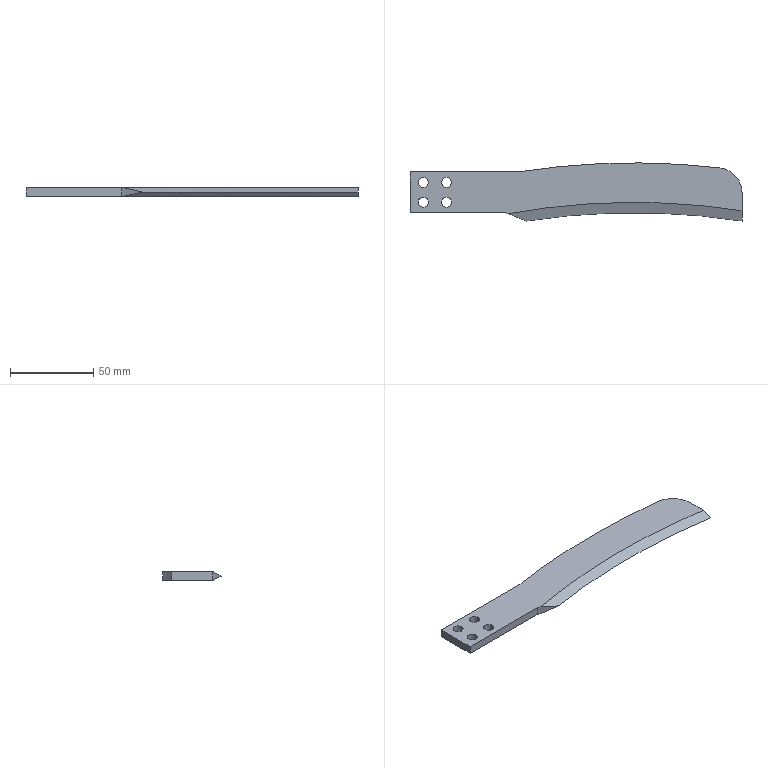Part | STEP file | Cut-off blade | 1 solid | 19 faces | box 200 x 35.06 x 5 mm | volume 25538 mm3 | cylinder 10 | plane 7 | cone 2 | commonest cylinder face diameters 6 x8 30 x1 900 x1
STEP:
#1=CARTESIAN_POINT('',(-51.,23.319,0.));
#2=VERTEX_POINT('',#1);
#3=CARTESIAN_POINT('',(-45.,23.319,0.));
#4=VERTEX_POINT('',#3);
#5=CARTESIAN_POINT('',(-48.,23.319,0.));
#6=DIRECTION('',(0.,0.,1.));
#7=DIRECTION('',(1.,0.,0.));
#8=AXIS2_PLACEMENT_3D('',#5,#6,#7);
#9=CIRCLE('',#8,3.);
#10=EDGE_CURVE('',#2,#4,#9,.T.);
#11=ORIENTED_EDGE('',*,*,#10,.F.);
#12=CARTESIAN_POINT('',(-51.,23.319,5.));
#13=VERTEX_POINT('',#12);
#14=CARTESIAN_POINT('',(-51.,23.319,0.));
#15=DIRECTION('',(0.,0.,1.));
#16=VECTOR('',#15,1000.);
#17=LINE('',#14,#16);
#18=EDGE_CURVE('',#2,#13,#17,.T.);
#19=ORIENTED_EDGE('',*,*,#18,.T.);
#20=CARTESIAN_POINT('',(-45.,23.319,5.));
#21=VERTEX_POINT('',#20);
#22=CARTESIAN_POINT('',(-48.,23.319,5.));
#23=DIRECTION('',(0.,0.,1.));
#24=DIRECTION('',(1.,0.,0.));
#25=AXIS2_PLACEMENT_3D('',#22,#23,#24);
#26=CIRCLE('',#25,3.);
#27=EDGE_CURVE('',#13,#21,#26,.T.);
#28=ORIENTED_EDGE('',*,*,#27,.T.);
#29=CARTESIAN_POINT('',(-45.,23.319,0.));
#30=DIRECTION('',(0.,0.,1.));
#31=VECTOR('',#30,1000.);
#32=LINE('',#29,#31);
#33=EDGE_CURVE('',#4,#21,#32,.T.);
#34=ORIENTED_EDGE('',*,*,#33,.F.);
#35=EDGE_LOOP('',(#11,#19,#28,#34));
#36=FACE_OUTER_BOUND('',#35,.T.);
#37=CARTESIAN_POINT('',(-48.,23.319,0.));
#38=DIRECTION('',(0.,0.,1.));
#39=DIRECTION('',(1.,0.,0.));
#40=AXIS2_PLACEMENT_3D('',#37,#38,#39);
#41=CYLINDRICAL_SURFACE('',#40,3.);
#42=ADVANCED_FACE('',(#36),#41,.F.);
#43=CARTESIAN_POINT('',(-51.,11.319,0.));
#44=VERTEX_POINT('',#43);
#45=CARTESIAN_POINT('',(-45.,11.319,0.));
#46=VERTEX_POINT('',#45);
#47=CARTESIAN_POINT('',(-48.,11.319,0.));
#48=DIRECTION('',(0.,0.,1.));
#49=DIRECTION('',(-1.,0.,0.));
#50=AXIS2_PLACEMENT_3D('',#47,#48,#49);
#51=CIRCLE('',#50,3.);
#52=EDGE_CURVE('',#44,#46,#51,.T.);
#53=ORIENTED_EDGE('',*,*,#52,.F.);
#54=CARTESIAN_POINT('',(-51.,11.319,5.));
#55=VERTEX_POINT('',#54);
#56=CARTESIAN_POINT('',(-51.,11.319,0.));
#57=DIRECTION('',(0.,0.,1.));
#58=VECTOR('',#57,1000.);
#59=LINE('',#56,#58);
#60=EDGE_CURVE('',#44,#55,#59,.T.);
#61=ORIENTED_EDGE('',*,*,#60,.T.);
#62=CARTESIAN_POINT('',(-45.,11.319,5.));
#63=VERTEX_POINT('',#62);
#64=CARTESIAN_POINT('',(-48.,11.319,5.));
#65=DIRECTION('',(0.,0.,1.));
#66=DIRECTION('',(-1.,0.,0.));
#67=AXIS2_PLACEMENT_3D('',#64,#65,#66);
#68=CIRCLE('',#67,3.);
#69=EDGE_CURVE('',#55,#63,#68,.T.);
#70=ORIENTED_EDGE('',*,*,#69,.T.);
#71=CARTESIAN_POINT('',(-45.,11.319,0.));
#72=DIRECTION('',(0.,0.,1.));
#73=VECTOR('',#72,1000.);
#74=LINE('',#71,#73);
#75=EDGE_CURVE('',#46,#63,#74,.T.);
#76=ORIENTED_EDGE('',*,*,#75,.F.);
#77=EDGE_LOOP('',(#53,#61,#70,#76));
#78=FACE_OUTER_BOUND('',#77,.T.);
#79=CARTESIAN_POINT('',(-48.,11.319,0.));
#80=DIRECTION('',(0.,0.,1.));
#81=DIRECTION('',(1.,0.,0.));
#82=AXIS2_PLACEMENT_3D('',#79,#80,#81);
#83=CYLINDRICAL_SURFACE('',#82,3.);
#84=ADVANCED_FACE('',(#78),#83,.F.);
#85=CARTESIAN_POINT('',(-65.,11.319,0.));
#86=VERTEX_POINT('',#85);
#87=CARTESIAN_POINT('',(-59.,11.319,0.));
#88=VERTEX_POINT('',#87);
#89=CARTESIAN_POINT('',(-62.,11.319,0.));
#90=DIRECTION('',(0.,0.,1.));
#91=DIRECTION('',(-1.,0.,0.));
#92=AXIS2_PLACEMENT_3D('',#89,#90,#91);
#93=CIRCLE('',#92,3.);
#94=EDGE_CURVE('',#86,#88,#93,.T.);
#95=ORIENTED_EDGE('',*,*,#94,.F.);
#96=CARTESIAN_POINT('',(-65.,11.319,5.));
#97=VERTEX_POINT('',#96);
#98=CARTESIAN_POINT('',(-65.,11.319,0.));
#99=DIRECTION('',(0.,0.,1.));
#100=VECTOR('',#99,1000.);
#101=LINE('',#98,#100);
#102=EDGE_CURVE('',#86,#97,#101,.T.);
#103=ORIENTED_EDGE('',*,*,#102,.T.);
#104=CARTESIAN_POINT('',(-59.,11.319,5.));
#105=VERTEX_POINT('',#104);
#106=CARTESIAN_POINT('',(-62.,11.319,5.));
#107=DIRECTION('',(0.,0.,1.));
#108=DIRECTION('',(-1.,0.,0.));
#109=AXIS2_PLACEMENT_3D('',#106,#107,#108);
#110=CIRCLE('',#109,3.);
#111=EDGE_CURVE('',#97,#105,#110,.T.);
#112=ORIENTED_EDGE('',*,*,#111,.T.);
#113=CARTESIAN_POINT('',(-59.,11.319,0.));
#114=DIRECTION('',(0.,0.,1.));
#115=VECTOR('',#114,1000.);
#116=LINE('',#113,#115);
#117=EDGE_CURVE('',#88,#105,#116,.T.);
#118=ORIENTED_EDGE('',*,*,#117,.F.);
#119=EDGE_LOOP('',(#95,#103,#112,#118));
#120=FACE_OUTER_BOUND('',#119,.T.);
#121=CARTESIAN_POINT('',(-62.,11.319,0.));
#122=DIRECTION('',(0.,0.,1.));
#123=DIRECTION('',(1.,0.,0.));
#124=AXIS2_PLACEMENT_3D('',#121,#122,#123);
#125=CYLINDRICAL_SURFACE('',#124,3.);
#126=ADVANCED_FACE('',(#120),#125,.F.);
#127=CARTESIAN_POINT('',(-65.,23.319,0.));
#128=VERTEX_POINT('',#127);
#129=CARTESIAN_POINT('',(-59.,23.319,0.));
#130=VERTEX_POINT('',#129);
#131=CARTESIAN_POINT('',(-62.,23.319,0.));
#132=DIRECTION('',(0.,0.,1.));
#133=DIRECTION('',(1.,0.,0.));
#134=AXIS2_PLACEMENT_3D('',#131,#132,#133);
#135=CIRCLE('',#134,3.);
#136=EDGE_CURVE('',#128,#130,#135,.T.);
#137=ORIENTED_EDGE('',*,*,#136,.F.);
#138=CARTESIAN_POINT('',(-65.,23.319,5.));
#139=VERTEX_POINT('',#138);
#140=CARTESIAN_POINT('',(-65.,23.319,0.));
#141=DIRECTION('',(0.,0.,1.));
#142=VECTOR('',#141,1000.);
#143=LINE('',#140,#142);
#144=EDGE_CURVE('',#128,#139,#143,.T.);
#145=ORIENTED_EDGE('',*,*,#144,.T.);
#146=CARTESIAN_POINT('',(-59.,23.319,5.));
#147=VERTEX_POINT('',#146);
#148=CARTESIAN_POINT('',(-62.,23.319,5.));
#149=DIRECTION('',(0.,0.,1.));
#150=DIRECTION('',(1.,0.,0.));
#151=AXIS2_PLACEMENT_3D('',#148,#149,#150);
#152=CIRCLE('',#151,3.);
#153=EDGE_CURVE('',#139,#147,#152,.T.);
#154=ORIENTED_EDGE('',*,*,#153,.T.);
#155=CARTESIAN_POINT('',(-59.,23.319,0.));
#156=DIRECTION('',(0.,0.,1.));
#157=VECTOR('',#156,1000.);
#158=LINE('',#155,#157);
#159=EDGE_CURVE('',#130,#147,#158,.T.);
#160=ORIENTED_EDGE('',*,*,#159,.F.);
#161=EDGE_LOOP('',(#137,#145,#154,#160));
#162=FACE_OUTER_BOUND('',#161,.T.);
#163=CARTESIAN_POINT('',(-62.,23.319,0.));
#164=DIRECTION('',(0.,0.,1.));
#165=DIRECTION('',(1.,0.,0.));
#166=AXIS2_PLACEMENT_3D('',#163,#164,#165);
#167=CYLINDRICAL_SURFACE('',#166,3.);
#168=ADVANCED_FACE('',(#162),#167,.F.);
#169=CARTESIAN_POINT('',(130.,6.262,0.));
#170=VERTEX_POINT('',#169);
#171=CARTESIAN_POINT('',(130.,17.177,0.));
#172=VERTEX_POINT('',#171);
#173=CARTESIAN_POINT('',(130.,0.,0.));
#174=DIRECTION('',(0.,1.,0.));
#175=VECTOR('',#174,1000.);
#176=LINE('',#173,#175);
#177=EDGE_CURVE('',#170,#172,#176,.T.);
#178=ORIENTED_EDGE('',*,*,#177,.T.);
#179=CARTESIAN_POINT('',(130.,17.177,5.));
#180=VERTEX_POINT('',#179);
#181=CARTESIAN_POINT('',(130.,17.177,5.));
#182=DIRECTION('',(0.,0.,1.));
#183=VECTOR('',#182,1000.);
#184=LINE('',#181,#183);
#185=EDGE_CURVE('',#172,#180,#184,.T.);
#186=ORIENTED_EDGE('',*,*,#185,.T.);
#187=CARTESIAN_POINT('',(130.,6.262,5.));
#188=VERTEX_POINT('',#187);
#189=CARTESIAN_POINT('',(130.,0.,5.));
#190=DIRECTION('',(0.,1.,0.));
#191=VECTOR('',#190,1000.);
#192=LINE('',#189,#191);
#193=EDGE_CURVE('',#188,#180,#192,.T.);
#194=ORIENTED_EDGE('',*,*,#193,.F.);
#195=CARTESIAN_POINT('',(130.,0.,2.5));
#196=VERTEX_POINT('',#195);
#197=CARTESIAN_POINT('',(130.,6.262,5.));
#198=CARTESIAN_POINT('',(130.,4.175,4.167));
#199=CARTESIAN_POINT('',(130.,2.087,3.333));
#200=CARTESIAN_POINT('',(130.,0.,2.5));
#201=B_SPLINE_CURVE_WITH_KNOTS('',3,(#197,#198,#199,#200),.UNSPECIFIED.,.F.,.F.,(4,4),(0.,0.006743),.UNSPECIFIED.);
#202=EDGE_CURVE('',#188,#196,#201,.T.);
#203=ORIENTED_EDGE('',*,*,#202,.T.);
#204=CARTESIAN_POINT('',(130.,0.,2.5));
#205=CARTESIAN_POINT('',(130.,2.087,1.667));
#206=CARTESIAN_POINT('',(130.,4.175,0.8335));
#207=CARTESIAN_POINT('',(130.,6.262,0.));
#208=B_SPLINE_CURVE_WITH_KNOTS('',3,(#204,#205,#206,#207),.UNSPECIFIED.,.F.,.F.,(4,4),(0.,0.006743),.UNSPECIFIED.);
#209=EDGE_CURVE('',#196,#170,#208,.T.);
#210=ORIENTED_EDGE('',*,*,#209,.T.);
#211=EDGE_LOOP('',(#178,#186,#194,#203,#210));
#212=FACE_OUTER_BOUND('',#211,.T.);
#213=CARTESIAN_POINT('',(130.,0.,5.));
#214=DIRECTION('',(-1.,0.,0.));
#215=DIRECTION('',(0.,0.,1.));
#216=AXIS2_PLACEMENT_3D('',#213,#214,#215);
#217=PLANE('',#216);
#218=ADVANCED_FACE('',(#212),#217,.F.);
#219=CARTESIAN_POINT('',(116.724,32.078,5.));
#220=VERTEX_POINT('',#219);
#221=CARTESIAN_POINT('',(-4.643,29.639,5.));
#222=VERTEX_POINT('',#221);
#223=CARTESIAN_POINT('',(65.,-414.94,5.));
#224=DIRECTION('',(0.,0.,1.));
#225=DIRECTION('',(-1.,0.,0.));
#226=AXIS2_PLACEMENT_3D('',#223,#224,#225);
#227=CIRCLE('',#226,450.);
#228=EDGE_CURVE('',#220,#222,#227,.T.);
#229=ORIENTED_EDGE('',*,*,#228,.F.);
#230=CARTESIAN_POINT('',(116.724,32.078,0.));
#231=VERTEX_POINT('',#230);
#232=CARTESIAN_POINT('',(116.724,32.078,5.));
#233=DIRECTION('',(0.,0.,-1.));
#234=VECTOR('',#233,1000.);
#235=LINE('',#232,#234);
#236=EDGE_CURVE('',#220,#231,#235,.T.);
#237=ORIENTED_EDGE('',*,*,#236,.T.);
#238=CARTESIAN_POINT('',(-4.643,29.639,0.));
#239=VERTEX_POINT('',#238);
#240=CARTESIAN_POINT('',(65.,-414.94,0.));
#241=DIRECTION('',(0.,0.,1.));
#242=DIRECTION('',(-1.,0.,0.));
#243=AXIS2_PLACEMENT_3D('',#240,#241,#242);
#244=CIRCLE('',#243,450.);
#245=EDGE_CURVE('',#231,#239,#244,.T.);
#246=ORIENTED_EDGE('',*,*,#245,.T.);
#247=CARTESIAN_POINT('',(-4.643,29.639,5.));
#248=DIRECTION('',(0.,0.,-1.));
#249=VECTOR('',#248,1000.);
#250=LINE('',#247,#249);
#251=EDGE_CURVE('',#222,#239,#250,.T.);
#252=ORIENTED_EDGE('',*,*,#251,.F.);
#253=EDGE_LOOP('',(#229,#237,#246,#252));
#254=FACE_OUTER_BOUND('',#253,.T.);
#255=CARTESIAN_POINT('',(65.,-414.94,5.));
#256=DIRECTION('',(0.,0.,-1.));
#257=DIRECTION('',(-1.,0.,0.));
#258=AXIS2_PLACEMENT_3D('',#255,#256,#257);
#259=CYLINDRICAL_SURFACE('',#258,450.);
#260=ADVANCED_FACE('',(#254),#259,.T.);
#261=CARTESIAN_POINT('',(-70.,29.639,0.));
#262=VERTEX_POINT('',#261);
#263=CARTESIAN_POINT('',(-4.643,29.639,0.));
#264=DIRECTION('',(-1.,0.,0.));
#265=VECTOR('',#264,1000.);
#266=LINE('',#263,#265);
#267=EDGE_CURVE('',#239,#262,#266,.T.);
#268=ORIENTED_EDGE('',*,*,#267,.T.);
#269=CARTESIAN_POINT('',(-70.,29.639,5.));
#270=VERTEX_POINT('',#269);
#271=CARTESIAN_POINT('',(-70.,29.639,5.));
#272=DIRECTION('',(0.,0.,-1.));
#273=VECTOR('',#272,1000.);
#274=LINE('',#271,#273);
#275=EDGE_CURVE('',#270,#262,#274,.T.);
#276=ORIENTED_EDGE('',*,*,#275,.F.);
#277=CARTESIAN_POINT('',(-4.643,29.639,5.));
#278=DIRECTION('',(-1.,0.,0.));
#279=VECTOR('',#278,1000.);
#280=LINE('',#277,#279);
#281=EDGE_CURVE('',#222,#270,#280,.T.);
#282=ORIENTED_EDGE('',*,*,#281,.F.);
#283=ORIENTED_EDGE('',*,*,#251,.T.);
#284=EDGE_LOOP('',(#268,#276,#282,#283));
#285=FACE_OUTER_BOUND('',#284,.T.);
#286=CARTESIAN_POINT('',(-4.643,29.639,5.));
#287=DIRECTION('',(0.,-1.,0.));
#288=DIRECTION('',(1.,0.,0.));
#289=AXIS2_PLACEMENT_3D('',#286,#287,#288);
#290=PLANE('',#289);
#291=ADVANCED_FACE('',(#285),#290,.F.);
#292=CARTESIAN_POINT('',(-70.,5.,0.));
#293=VERTEX_POINT('',#292);
#294=CARTESIAN_POINT('',(-70.,29.639,0.));
#295=DIRECTION('',(0.,-1.,0.));
#296=VECTOR('',#295,1000.);
#297=LINE('',#294,#296);
#298=EDGE_CURVE('',#262,#293,#297,.T.);
#299=ORIENTED_EDGE('',*,*,#298,.T.);
#300=CARTESIAN_POINT('',(-70.,5.,5.));
#301=VERTEX_POINT('',#300);
#302=CARTESIAN_POINT('',(-70.,5.,0.));
#303=DIRECTION('',(0.,0.,1.));
#304=VECTOR('',#303,1000.);
#305=LINE('',#302,#304);
#306=EDGE_CURVE('',#293,#301,#305,.T.);
#307=ORIENTED_EDGE('',*,*,#306,.T.);
#308=CARTESIAN_POINT('',(-70.,29.639,5.));
#309=DIRECTION('',(0.,-1.,0.));
#310=VECTOR('',#309,1000.);
#311=LINE('',#308,#310);
#312=EDGE_CURVE('',#270,#301,#311,.T.);
#313=ORIENTED_EDGE('',*,*,#312,.F.);
#314=ORIENTED_EDGE('',*,*,#275,.T.);
#315=EDGE_LOOP('',(#299,#307,#313,#314));
#316=FACE_OUTER_BOUND('',#315,.T.);
#317=CARTESIAN_POINT('',(-70.,29.639,5.));
#318=DIRECTION('',(1.,0.,0.));
#319=DIRECTION('',(0.,0.,-1.));
#320=AXIS2_PLACEMENT_3D('',#317,#318,#319);
#321=PLANE('',#320);
#322=ADVANCED_FACE('',(#316),#321,.F.);
#323=CARTESIAN_POINT('',(-48.,23.319,5.));
#324=DIRECTION('',(0.,0.,1.));
#325=DIRECTION('',(1.,0.,0.));
#326=AXIS2_PLACEMENT_3D('',#323,#324,#325);
#327=CIRCLE('',#326,3.);
#328=EDGE_CURVE('',#21,#13,#327,.T.);
#329=ORIENTED_EDGE('',*,*,#328,.F.);
#330=ORIENTED_EDGE('',*,*,#27,.F.);
#331=EDGE_LOOP('',(#329,#330));
#332=FACE_BOUND('',#331,.T.);
#333=CARTESIAN_POINT('',(-48.,11.319,5.));
#334=DIRECTION('',(0.,0.,1.));
#335=DIRECTION('',(-1.,0.,0.));
#336=AXIS2_PLACEMENT_3D('',#333,#334,#335);
#337=CIRCLE('',#336,3.);
#338=EDGE_CURVE('',#63,#55,#337,.T.);
#339=ORIENTED_EDGE('',*,*,#338,.F.);
#340=ORIENTED_EDGE('',*,*,#69,.F.);
#341=EDGE_LOOP('',(#339,#340));
#342=FACE_BOUND('',#341,.T.);
#343=CARTESIAN_POINT('',(-62.,11.319,5.));
#344=DIRECTION('',(0.,0.,1.));
#345=DIRECTION('',(-1.,0.,0.));
#346=AXIS2_PLACEMENT_3D('',#343,#344,#345);
#347=CIRCLE('',#346,3.);
#348=EDGE_CURVE('',#105,#97,#347,.T.);
#349=ORIENTED_EDGE('',*,*,#348,.F.);
#350=ORIENTED_EDGE('',*,*,#111,.F.);
#351=EDGE_LOOP('',(#349,#350));
#352=FACE_BOUND('',#351,.T.);
#353=CARTESIAN_POINT('',(-62.,23.319,5.));
#354=DIRECTION('',(0.,0.,1.));
#355=DIRECTION('',(1.,0.,0.));
#356=AXIS2_PLACEMENT_3D('',#353,#354,#355);
#357=CIRCLE('',#356,3.);
#358=EDGE_CURVE('',#147,#139,#357,.T.);
#359=ORIENTED_EDGE('',*,*,#358,.F.);
#360=ORIENTED_EDGE('',*,*,#153,.F.);
#361=EDGE_LOOP('',(#359,#360));
#362=FACE_BOUND('',#361,.T.);
#363=ORIENTED_EDGE('',*,*,#193,.T.);
#364=CARTESIAN_POINT('',(115.,17.177,5.));
#365=DIRECTION('',(0.,0.,1.));
#366=DIRECTION('',(-1.,0.,0.));
#367=AXIS2_PLACEMENT_3D('',#364,#365,#366);
#368=CIRCLE('',#367,15.);
#369=EDGE_CURVE('',#180,#220,#368,.T.);
#370=ORIENTED_EDGE('',*,*,#369,.T.);
#371=ORIENTED_EDGE('',*,*,#228,.T.);
#372=ORIENTED_EDGE('',*,*,#281,.T.);
#373=ORIENTED_EDGE('',*,*,#312,.T.);
#374=CARTESIAN_POINT('',(-12.375,5.,5.));
#375=VERTEX_POINT('',#374);
#376=CARTESIAN_POINT('',(0.,5.,5.));
#377=DIRECTION('',(-1.,0.,0.));
#378=VECTOR('',#377,1000.);
#379=LINE('',#376,#378);
#380=EDGE_CURVE('',#375,#301,#379,.T.);
#381=ORIENTED_EDGE('',*,*,#380,.F.);
#382=CARTESIAN_POINT('',(-10.953,4.425,5.));
#383=VERTEX_POINT('',#382);
#384=CARTESIAN_POINT('',(199.999,-80.805,5.));
#385=DIRECTION('',(0.9272,-0.3746,0.));
#386=VECTOR('',#385,1000.);
#387=LINE('',#384,#386);
#388=EDGE_CURVE('',#375,#383,#387,.T.);
#389=ORIENTED_EDGE('',*,*,#388,.T.);
#390=CARTESIAN_POINT('',(65.,-414.94,5.));
#391=DIRECTION('',(0.,0.,-1.));
#392=DIRECTION('',(-1.,0.,0.));
#393=AXIS2_PLACEMENT_3D('',#390,#391,#392);
#394=CIRCLE('',#393,426.188);
#395=EDGE_CURVE('',#383,#188,#394,.T.);
#396=ORIENTED_EDGE('',*,*,#395,.T.);
#397=EDGE_LOOP('',(#363,#370,#371,#372,#373,#381,#389,#396));
#398=FACE_OUTER_BOUND('',#397,.T.);
#399=CARTESIAN_POINT('',(65.,-414.94,5.));
#400=DIRECTION('',(0.,0.,-1.));
#401=DIRECTION('',(-1.,0.,0.));
#402=AXIS2_PLACEMENT_3D('',#399,#400,#401);
#403=PLANE('',#402);
#404=ADVANCED_FACE('',(#332,#342,#352,#362,#398),#403,.F.);
#405=CARTESIAN_POINT('',(-48.,23.319,0.));
#406=DIRECTION('',(0.,0.,1.));
#407=DIRECTION('',(1.,0.,0.));
#408=AXIS2_PLACEMENT_3D('',#405,#406,#407);
#409=CIRCLE('',#408,3.);
#410=EDGE_CURVE('',#4,#2,#409,.T.);
#411=ORIENTED_EDGE('',*,*,#410,.T.);
#412=ORIENTED_EDGE('',*,*,#10,.T.);
#413=EDGE_LOOP('',(#411,#412));
#414=FACE_BOUND('',#413,.T.);
#415=CARTESIAN_POINT('',(-48.,11.319,0.));
#416=DIRECTION('',(0.,0.,1.));
#417=DIRECTION('',(-1.,0.,0.));
#418=AXIS2_PLACEMENT_3D('',#415,#416,#417);
#419=CIRCLE('',#418,3.);
#420=EDGE_CURVE('',#46,#44,#419,.T.);
#421=ORIENTED_EDGE('',*,*,#420,.T.);
#422=ORIENTED_EDGE('',*,*,#52,.T.);
#423=EDGE_LOOP('',(#421,#422));
#424=FACE_BOUND('',#423,.T.);
#425=CARTESIAN_POINT('',(-62.,11.319,0.));
#426=DIRECTION('',(0.,0.,1.));
#427=DIRECTION('',(-1.,0.,0.));
#428=AXIS2_PLACEMENT_3D('',#425,#426,#427);
#429=CIRCLE('',#428,3.);
#430=EDGE_CURVE('',#88,#86,#429,.T.);
#431=ORIENTED_EDGE('',*,*,#430,.T.);
#432=ORIENTED_EDGE('',*,*,#94,.T.);
#433=EDGE_LOOP('',(#431,#432));
#434=FACE_BOUND('',#433,.T.);
#435=CARTESIAN_POINT('',(-62.,23.319,0.));
#436=DIRECTION('',(0.,0.,1.));
#437=DIRECTION('',(1.,0.,0.));
#438=AXIS2_PLACEMENT_3D('',#435,#436,#437);
#439=CIRCLE('',#438,3.);
#440=EDGE_CURVE('',#130,#128,#439,.T.);
#441=ORIENTED_EDGE('',*,*,#440,.T.);
#442=ORIENTED_EDGE('',*,*,#136,.T.);
#443=EDGE_LOOP('',(#441,#442));
#444=FACE_BOUND('',#443,.T.);
#445=ORIENTED_EDGE('',*,*,#245,.F.);
#446=CARTESIAN_POINT('',(115.,17.177,0.));
#447=DIRECTION('',(0.,0.,-1.));
#448=DIRECTION('',(-1.,0.,0.));
#449=AXIS2_PLACEMENT_3D('',#446,#447,#448);
#450=CIRCLE('',#449,15.);
#451=EDGE_CURVE('',#231,#172,#450,.T.);
#452=ORIENTED_EDGE('',*,*,#451,.T.);
#453=ORIENTED_EDGE('',*,*,#177,.F.);
#454=CARTESIAN_POINT('',(-10.953,4.425,0.));
#455=VERTEX_POINT('',#454);
#456=CARTESIAN_POINT('',(65.,-414.94,0.));
#457=DIRECTION('',(0.,0.,1.));
#458=DIRECTION('',(-1.,0.,0.));
#459=AXIS2_PLACEMENT_3D('',#456,#457,#458);
#460=CIRCLE('',#459,426.188);
#461=EDGE_CURVE('',#170,#455,#460,.T.);
#462=ORIENTED_EDGE('',*,*,#461,.T.);
#463=CARTESIAN_POINT('',(-12.375,5.,0.));
#464=VERTEX_POINT('',#463);
#465=CARTESIAN_POINT('',(-12.375,5.,0.));
#466=DIRECTION('',(-0.9272,0.3746,0.));
#467=VECTOR('',#466,1000.);
#468=LINE('',#465,#467);
#469=EDGE_CURVE('',#455,#464,#468,.T.);
#470=ORIENTED_EDGE('',*,*,#469,.T.);
#471=CARTESIAN_POINT('',(0.,5.,0.));
#472=DIRECTION('',(-1.,0.,0.));
#473=VECTOR('',#472,1000.);
#474=LINE('',#471,#473);
#475=EDGE_CURVE('',#464,#293,#474,.T.);
#476=ORIENTED_EDGE('',*,*,#475,.T.);
#477=ORIENTED_EDGE('',*,*,#298,.F.);
#478=ORIENTED_EDGE('',*,*,#267,.F.);
#479=EDGE_LOOP('',(#445,#452,#453,#462,#470,#476,#477,#478));
#480=FACE_OUTER_BOUND('',#479,.T.);
#481=CARTESIAN_POINT('',(65.,-414.94,0.));
#482=DIRECTION('',(0.,0.,-1.));
#483=DIRECTION('',(-1.,0.,0.));
#484=AXIS2_PLACEMENT_3D('',#481,#482,#483);
#485=PLANE('',#484);
#486=ADVANCED_FACE('',(#414,#424,#434,#444,#480),#485,.T.);
#487=ORIENTED_EDGE('',*,*,#475,.F.);
#488=CARTESIAN_POINT('',(-12.375,5.,4.496));
#489=DIRECTION('',(0.,0.,1.));
#490=VECTOR('',#489,1000.);
#491=LINE('',#488,#490);
#492=EDGE_CURVE('',#464,#375,#491,.T.);
#493=ORIENTED_EDGE('',*,*,#492,.T.);
#494=ORIENTED_EDGE('',*,*,#380,.T.);
#495=ORIENTED_EDGE('',*,*,#306,.F.);
#496=EDGE_LOOP('',(#487,#493,#494,#495));
#497=FACE_OUTER_BOUND('',#496,.T.);
#498=CARTESIAN_POINT('',(0.,5.,0.));
#499=DIRECTION('',(0.,1.,0.));
#500=DIRECTION('',(-1.,0.,0.));
#501=AXIS2_PLACEMENT_3D('',#498,#499,#500);
#502=PLANE('',#501);
#503=ADVANCED_FACE('',(#497),#502,.F.);
#504=ORIENTED_EDGE('',*,*,#395,.F.);
#505=CARTESIAN_POINT('',(0.,0.,2.5));
#506=VERTEX_POINT('',#505);
#507=CARTESIAN_POINT('',(-10.953,4.425,5.));
#508=CARTESIAN_POINT('',(-7.305,2.951,4.151));
#509=CARTESIAN_POINT('',(-3.654,1.476,3.318));
#510=CARTESIAN_POINT('',(0.,0.,2.5));
#511=B_SPLINE_CURVE_WITH_KNOTS('',3,(#507,#508,#509,#510),.UNSPECIFIED.,.F.,.F.,(4,4),(0.,0.01207),.UNSPECIFIED.);
#512=EDGE_CURVE('',#383,#506,#511,.T.);
#513=ORIENTED_EDGE('',*,*,#512,.T.);
#514=CARTESIAN_POINT('',(65.,-414.94,2.5));
#515=DIRECTION('',(0.,0.,1.));
#516=DIRECTION('',(-1.,0.,0.));
#517=AXIS2_PLACEMENT_3D('',#514,#515,#516);
#518=CIRCLE('',#517,420.);
#519=EDGE_CURVE('',#196,#506,#518,.T.);
#520=ORIENTED_EDGE('',*,*,#519,.F.);
#521=ORIENTED_EDGE('',*,*,#202,.F.);
#522=EDGE_LOOP('',(#504,#513,#520,#521));
#523=FACE_OUTER_BOUND('',#522,.T.);
#524=CARTESIAN_POINT('',(65.,-414.94,5.));
#525=DIRECTION('',(0.,0.,1.));
#526=DIRECTION('',(1.,0.,0.));
#527=AXIS2_PLACEMENT_3D('',#524,#525,#526);
#528=CONICAL_SURFACE('',#527,426.188,1.187);
#529=ADVANCED_FACE('',(#523),#528,.F.);
#530=ORIENTED_EDGE('',*,*,#519,.T.);
#531=CARTESIAN_POINT('',(0.,0.,2.5));
#532=CARTESIAN_POINT('',(-3.654,1.476,1.682));
#533=CARTESIAN_POINT('',(-7.305,2.951,0.8486));
#534=CARTESIAN_POINT('',(-10.953,4.425,0.));
#535=B_SPLINE_CURVE_WITH_KNOTS('',3,(#531,#532,#533,#534),.UNSPECIFIED.,.F.,.F.,(4,4),(0.,0.01207),.UNSPECIFIED.);
#536=EDGE_CURVE('',#506,#455,#535,.T.);
#537=ORIENTED_EDGE('',*,*,#536,.T.);
#538=ORIENTED_EDGE('',*,*,#461,.F.);
#539=ORIENTED_EDGE('',*,*,#209,.F.);
#540=EDGE_LOOP('',(#530,#537,#538,#539));
#541=FACE_OUTER_BOUND('',#540,.T.);
#542=CARTESIAN_POINT('',(65.,-414.94,2.5));
#543=DIRECTION('',(0.,0.,-1.));
#544=DIRECTION('',(-1.,0.,0.));
#545=AXIS2_PLACEMENT_3D('',#542,#543,#544);
#546=CONICAL_SURFACE('',#545,420.,1.187);
#547=ADVANCED_FACE('',(#541),#546,.F.);
#548=ORIENTED_EDGE('',*,*,#144,.F.);
#549=ORIENTED_EDGE('',*,*,#440,.F.);
#550=ORIENTED_EDGE('',*,*,#159,.T.);
#551=ORIENTED_EDGE('',*,*,#358,.T.);
#552=EDGE_LOOP('',(#548,#549,#550,#551));
#553=FACE_OUTER_BOUND('',#552,.T.);
#554=CARTESIAN_POINT('',(-62.,23.319,0.));
#555=DIRECTION('',(0.,0.,1.));
#556=DIRECTION('',(1.,0.,0.));
#557=AXIS2_PLACEMENT_3D('',#554,#555,#556);
#558=CYLINDRICAL_SURFACE('',#557,3.);
#559=ADVANCED_FACE('',(#553),#558,.F.);
#560=ORIENTED_EDGE('',*,*,#102,.F.);
#561=ORIENTED_EDGE('',*,*,#430,.F.);
#562=ORIENTED_EDGE('',*,*,#117,.T.);
#563=ORIENTED_EDGE('',*,*,#348,.T.);
#564=EDGE_LOOP('',(#560,#561,#562,#563));
#565=FACE_OUTER_BOUND('',#564,.T.);
#566=CARTESIAN_POINT('',(-62.,11.319,0.));
#567=DIRECTION('',(0.,0.,1.));
#568=DIRECTION('',(1.,0.,0.));
#569=AXIS2_PLACEMENT_3D('',#566,#567,#568);
#570=CYLINDRICAL_SURFACE('',#569,3.);
#571=ADVANCED_FACE('',(#565),#570,.F.);
#572=ORIENTED_EDGE('',*,*,#60,.F.);
#573=ORIENTED_EDGE('',*,*,#420,.F.);
#574=ORIENTED_EDGE('',*,*,#75,.T.);
#575=ORIENTED_EDGE('',*,*,#338,.T.);
#576=EDGE_LOOP('',(#572,#573,#574,#575));
#577=FACE_OUTER_BOUND('',#576,.T.);
#578=CARTESIAN_POINT('',(-48.,11.319,0.));
#579=DIRECTION('',(0.,0.,1.));
#580=DIRECTION('',(1.,0.,0.));
#581=AXIS2_PLACEMENT_3D('',#578,#579,#580);
#582=CYLINDRICAL_SURFACE('',#581,3.);
#583=ADVANCED_FACE('',(#577),#582,.F.);
#584=ORIENTED_EDGE('',*,*,#18,.F.);
#585=ORIENTED_EDGE('',*,*,#410,.F.);
#586=ORIENTED_EDGE('',*,*,#33,.T.);
#587=ORIENTED_EDGE('',*,*,#328,.T.);
#588=EDGE_LOOP('',(#584,#585,#586,#587));
#589=FACE_OUTER_BOUND('',#588,.T.);
#590=CARTESIAN_POINT('',(-48.,23.319,0.));
#591=DIRECTION('',(0.,0.,1.));
#592=DIRECTION('',(1.,0.,0.));
#593=AXIS2_PLACEMENT_3D('',#590,#591,#592);
#594=CYLINDRICAL_SURFACE('',#593,3.);
#595=ADVANCED_FACE('',(#589),#594,.F.);
#596=ORIENTED_EDGE('',*,*,#469,.F.);
#597=ORIENTED_EDGE('',*,*,#536,.F.);
#598=ORIENTED_EDGE('',*,*,#512,.F.);
#599=ORIENTED_EDGE('',*,*,#388,.F.);
#600=ORIENTED_EDGE('',*,*,#492,.F.);
#601=EDGE_LOOP('',(#596,#597,#598,#599,#600));
#602=FACE_OUTER_BOUND('',#601,.T.);
#603=CARTESIAN_POINT('',(-12.375,5.,0.));
#604=DIRECTION('',(-0.3746,-0.9272,0.));
#605=DIRECTION('',(0.,0.,-1.));
#606=AXIS2_PLACEMENT_3D('',#603,#604,#605);
#607=PLANE('',#606);
#608=ADVANCED_FACE('',(#602),#607,.T.);
#609=ORIENTED_EDGE('',*,*,#369,.F.);
#610=ORIENTED_EDGE('',*,*,#185,.F.);
#611=ORIENTED_EDGE('',*,*,#451,.F.);
#612=ORIENTED_EDGE('',*,*,#236,.F.);
#613=EDGE_LOOP('',(#609,#610,#611,#612));
#614=FACE_OUTER_BOUND('',#613,.T.);
#615=CARTESIAN_POINT('',(115.,17.177,5.));
#616=DIRECTION('',(0.,0.,-1.));
#617=DIRECTION('',(-1.,0.,0.));
#618=AXIS2_PLACEMENT_3D('',#615,#616,#617);
#619=CYLINDRICAL_SURFACE('',#618,15.);
#620=ADVANCED_FACE('',(#614),#619,.T.);
#621=CLOSED_SHELL('',(#42,#84,#126,#168,#218,#260,#291,#322,#404,#486,#503,#529,#547,#559,#571,#583,#595,#608,#620));
#622=MANIFOLD_SOLID_BREP('',#621);
#623=CARTESIAN_POINT('',(0.,0.,0.));
#624=DIRECTION('',(0.,0.,1.));
#625=DIRECTION('',(1.,0.,0.));
#626=AXIS2_PLACEMENT_3D('',#623,#624,#625);
#627=(LENGTH_UNIT()NAMED_UNIT(*)SI_UNIT(.MILLI.,.METRE.));
#628=UNCERTAINTY_MEASURE_WITH_UNIT(LENGTH_MEASURE(0.00001),#627,'','');
#629=(NAMED_UNIT(*)PLANE_ANGLE_UNIT()SI_UNIT($,.RADIAN.));
#630=(NAMED_UNIT(*)SI_UNIT($,.STERADIAN.)SOLID_ANGLE_UNIT());
#631=(GEOMETRIC_REPRESENTATION_CONTEXT(3)GLOBAL_UNCERTAINTY_ASSIGNED_CONTEXT((#628))GLOBAL_UNIT_ASSIGNED_CONTEXT((#627,#629,#630))REPRESENTATION_CONTEXT('',''));
#632=ADVANCED_BREP_SHAPE_REPRESENTATION('',(#622,#626),#631);